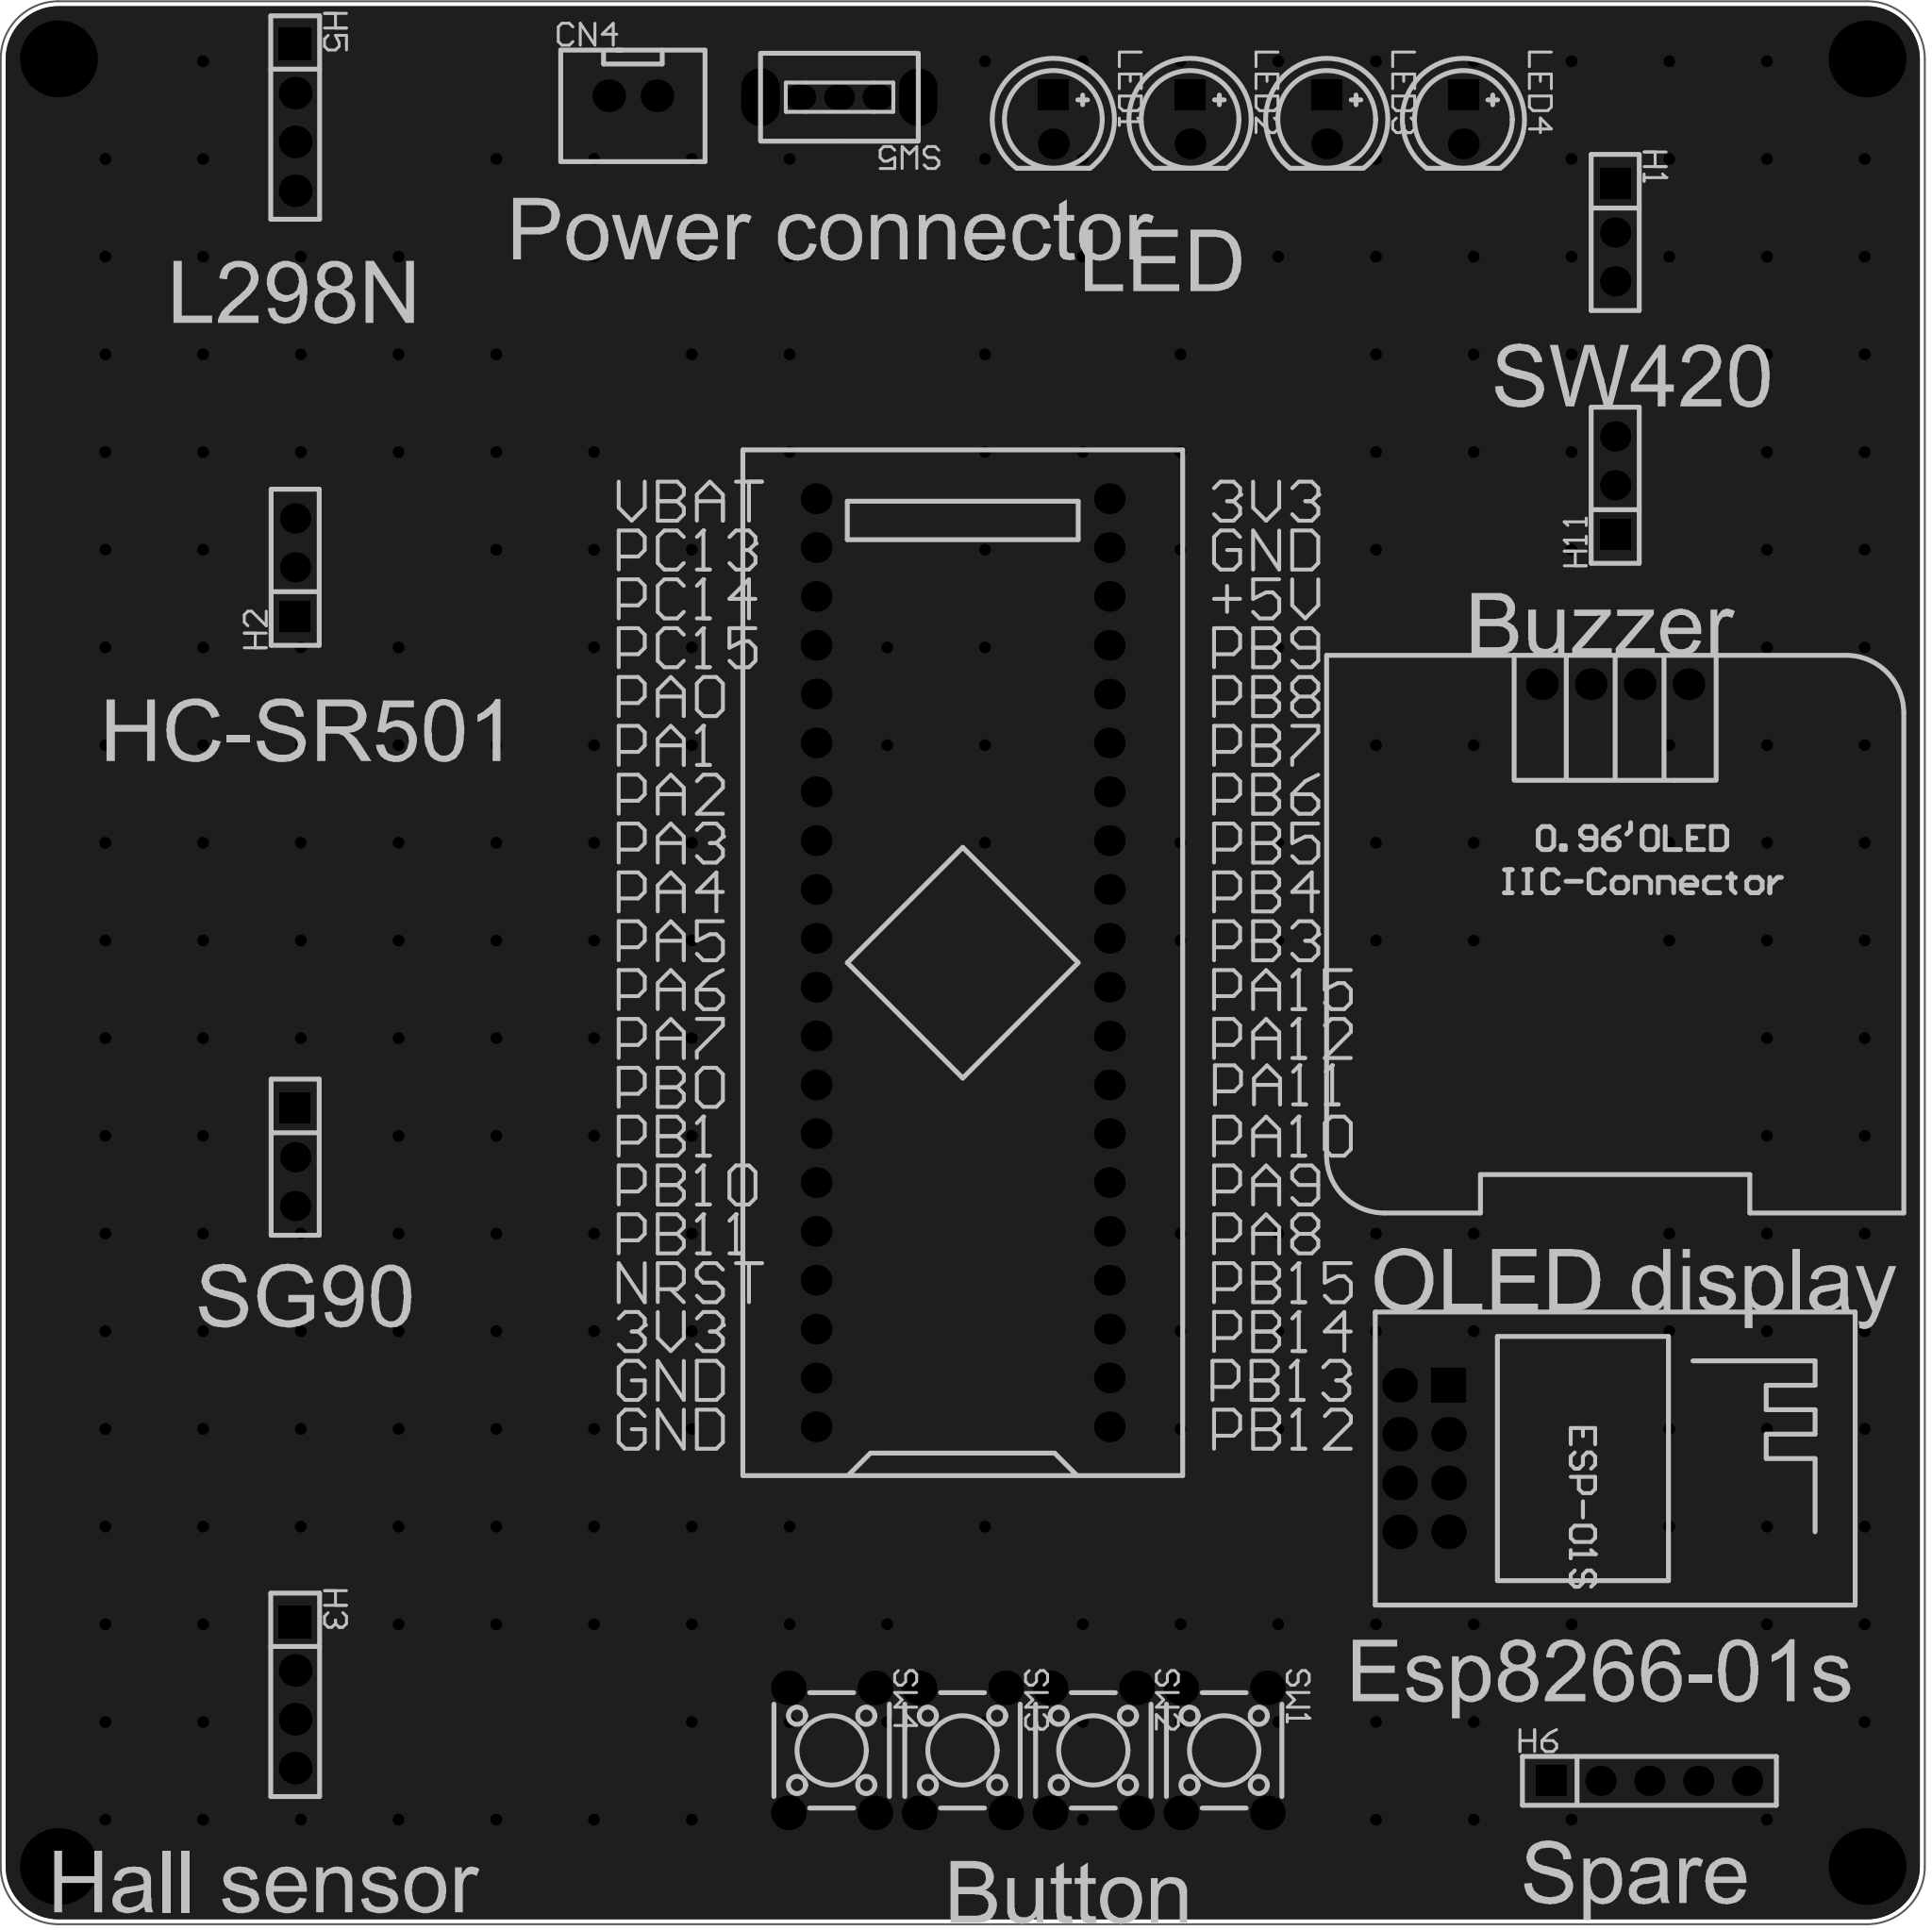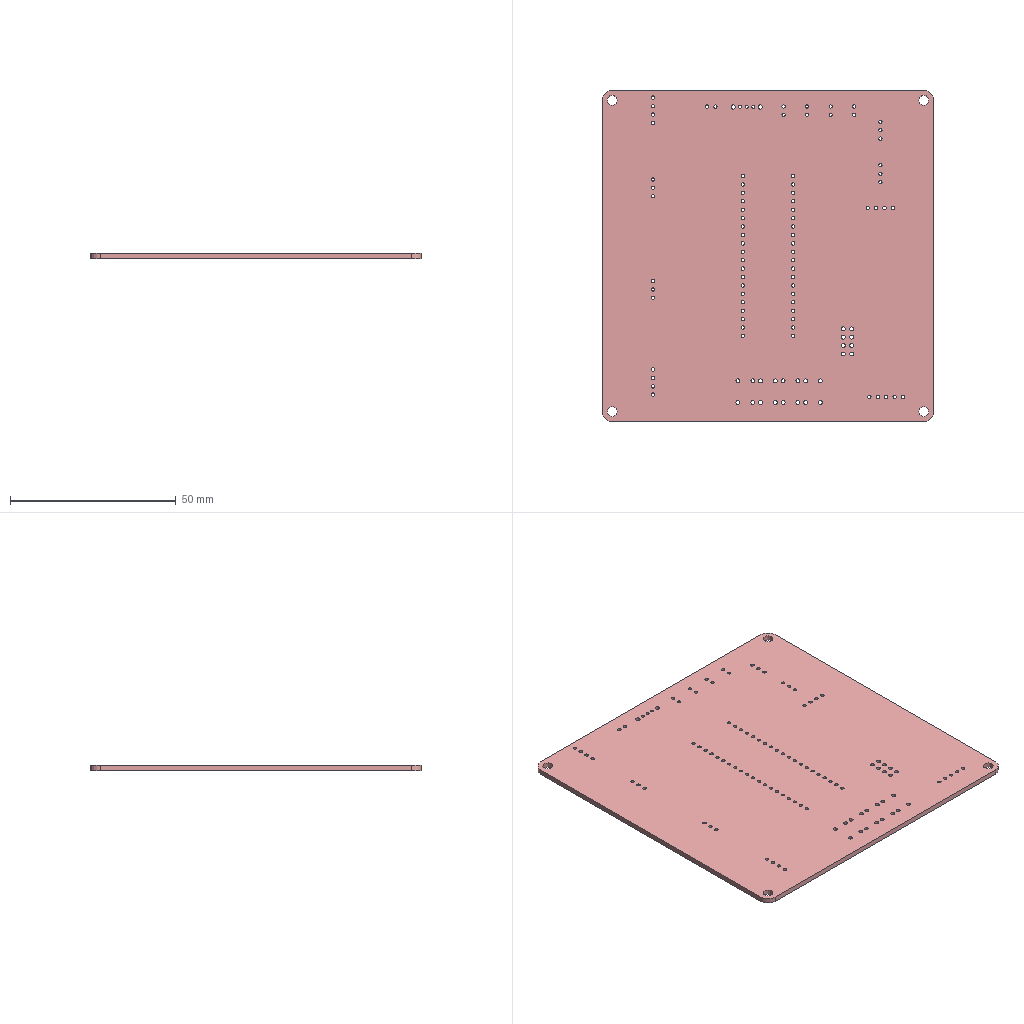Circuit board layout | Altium Designer | box 100 x 100 x 1.6 mm
Layer stack:
# Altium Designer layer stack of  (unit mm; dielectric type: 0 none, 1 core, 2 prepreg, 3 surface material)
index,name,kind,layer,copper_thickness_mm,dielectric_type,dielectric_thickness_mm,dielectric_material,dielectric_constant
0,Top Paste Mask Layer,other,,,,,,
1,Top Silkscreen Layer,other,,,,,,
2,Top Solder Mask Layer,dielectric,,,3,0.01,,3.3
3,Top Layer,copper,Top Layer,0.035,,,,
4,Dielectric1,dielectric,,,3,1.51,FR4,4.5
5,Bottom Layer,copper,Bottom Layer,0.035,,,,
6,Bottom Solder Mask Layer,dielectric,,,3,0.01,,3.3
7,Bottom Silkscreen Layer,other,,,,,,
8,Bottom Paste Mask Layer,other,,,,,,
# drill layer pairs: low layer,high layer
drill_pair,Top Layer,Bottom Layer
Part placement:
Designator,Comment,Layer,Footprint,Center-X(mm),Center-Y(mm),Rotation
U1,STM32F103C8T6-Card,TopLayer,CONN-TH_L53.3-W22.9_STM32F103C8T6-CARD,141.351,130.937,90
U2,ESP-01S,TopLayer,WIFIM-TH_ESP-01S,165.328,105.154,270
OLED1,,TopLayer,0.96OLED_4P,175.26,145.422,0
SW1,,TopLayer,SW-TH_4P-L6.0-W6.0-P4.50-LS6.5,154.936,89.979,270
SW2,,TopLayer,SW-TH_4P-L6.0-W6.0-P4.50-LS6.5,148.136,89.979,270
SW3,,TopLayer,SW-TH_4P-L6.0-W6.0-P4.50-LS6.5,141.337,89.979,270
SW4,,TopLayer,SW-TH_4P-L6.0-W6.0-P4.50-LS6.5,134.537,89.979,270
H11,,TopLayer,HDR-TH_3P-P2.54-V-F,175.26,155.767,90
H12,,TopLayer,HDR-TH_3P-P2.54-V-F,106.655,120.825,270
CN4,XH2.54*2P_through-hole,TopLayer,CONN-TH_2P-P2.50-XH2.54-2P,124.206,176.022,0
SW5,,TopLayer,拨动开关,134.94,175.947,180
H1,,TopLayer,HDR-TH_3P-P2.54-V-F,175.26,168.912,270
H2,,TopLayer,HDR-TH_3P-P2.54-V-F,106.655,151.502,90
H3,,TopLayer,HDR-TH_4P-P2.54-V-F,106.655,92.866,270
H5,,TopLayer,HDR-TH_4P-P2.54-V-F,106.655,174.889,270
LED1,,TopLayer,LED-TH_5mm,146.059,174.792,270
LED2,,TopLayer,LED-TH_5mm,153.163,174.792,270
LED3,,TopLayer,LED-TH_5mm,160.267,174.792,270
LED4,,TopLayer,LED-TH_5mm,167.371,174.792,270
H6,,TopLayer,HDR-TH_5P-P2.54-V-F,177.038,88.392,0
Pad and via stacks:
# Altium Designer via and pad stacks of  (unit mm). Each distinct definition once, with the count of objects using it.
# via: kind,start_layer,end_layer,hole_mm,diameter_mm,mode(0 simple;1 top-mid-bottom;2 full stack),diameter_per_layer,count,example_net
# pad: kind,layer,hole_mm,hole_type(0 round;1 square;2 slot),plating,top_size,top_shape(1 round;2 rect;3 octagon;9 rounded rect),mid_size,bottom_size,mode,footprint,size_per_layer,count,example
pad,Multi-Layer,3,0,plated,4x4,1,4x4,4x4,0,,,4,1
pad,Multi-Layer,1,0,plated,1.6x1.6,1,1.6x1.6,1.6x1.6,0,CONN-TH_L53.3-W22.9_STM32F103C8T6-CARD,,40,U1.1
pad,Multi-Layer,1.2,0,plated,1.8x1.8,2,1.8x1.8,1.8x1.8,0,WIFIM-TH_ESP-01S,,1,U2.1
pad,Multi-Layer,1.2,0,plated,1.8x1.8,1,1.8x1.8,1.8x1.8,0,WIFIM-TH_ESP-01S,,7,U2.2
pad,Multi-Layer,1,0,plated,1.65x1.65,1,1.65x1.65,1.65x1.65,0,0.96OLED_4P,,4,OLED1.4
pad,Multi-Layer,1.2,0,plated,1.8x1.8,1,1.8x1.8,1.8x1.8,0,SW-TH_4P-L6.0-W6.0-P4.50-LS6.5,,16,SW1.1
pad,Multi-Layer,1.02,0,plated,1.575x1.575,1,1.575x1.575,1.575x1.575,0,HDR-TH_3P-P2.54-V-F,,8,H11.3
pad,Multi-Layer,1.02,0,plated,1.575x1.575,2,1.575x1.575,1.575x1.575,0,HDR-TH_3P-P2.54-V-F,,4,H11.1
pad,Multi-Layer,1.05,0,plated,1.7x1.7,1,1.7x1.7,1.7x1.7,0,CONN-TH_2P-P2.50-XH2.54-2P,,2,CN4.2
pad,Multi-Layer,0.8992,0,plated,1.6x1.3,1,1.6x1.3,1.6x1.3,0,\u00B2\u00A6\u00B6\u00AF\u00BF\u00AA\u00B9\u00D8,,3,SW5.1
pad,Multi-Layer,1.3,0,plated,3x1.999,1,3x1.999,3x1.999,0,\u00B2\u00A6\u00B6\u00AF\u00BF\u00AA\u00B9\u00D8,,2,SW5.4
pad,Multi-Layer,1.1,0,plated,1.7x1.7,2,1.7x1.7,1.7x1.7,0,HDR-TH_4P-P2.54-V-F,,2,H3.1
pad,Multi-Layer,1.1,0,plated,1.7x1.7,1,1.7x1.7,1.7x1.7,0,HDR-TH_4P-P2.54-V-F,,6,H3.2
pad,Multi-Layer,1,0,plated,1.6x1.6,2,1.6x1.6,1.6x1.6,0,LED-TH_5mm,,4,LED1.1
pad,Multi-Layer,1,0,plated,1.6x1.6,1,1.6x1.6,1.6x1.6,0,LED-TH_5mm,,4,LED1.2
pad,Multi-Layer,1.02,0,plated,1.575x1.575,1,1.575x1.575,1.575x1.575,0,HDR-TH_5P-P2.54-V-F,,4,H6.5
pad,Multi-Layer,1.02,0,plated,1.575x1.575,2,1.575x1.575,1.575x1.575,0,HDR-TH_5P-P2.54-V-F,,1,H6.1
via,Top Layer,Bottom Layer,0.3048,0.61,0,,242,GND
Copper pours:
name,layer,net,type(0 solid;1 hatched;2 none)
Bottom Layer-GND,Bottom Layer,GND,0
Top Layer-GND,Top Layer,GND,0